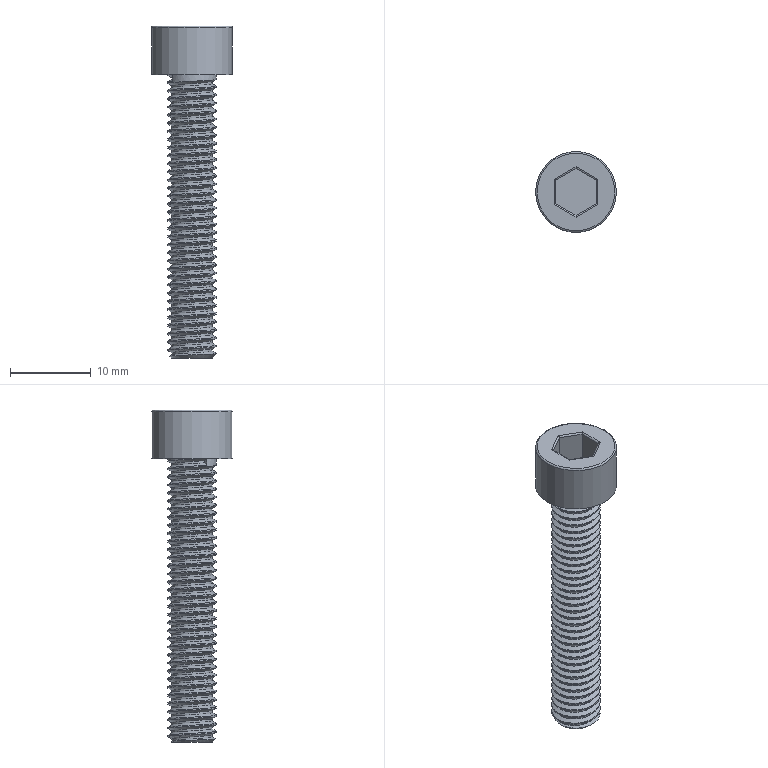Part | STEP file | Tube feed_id1034_x_t | 1 solid | 26 faces | box 10 x 10 x 41 mm | volume 1187 mm3 | plane 12 | cylinder 9 | spline 3 | cone 1 | torus 1 | commonest cylinder face diameters 0.4 x6 5 x1 6 x1 10 x1